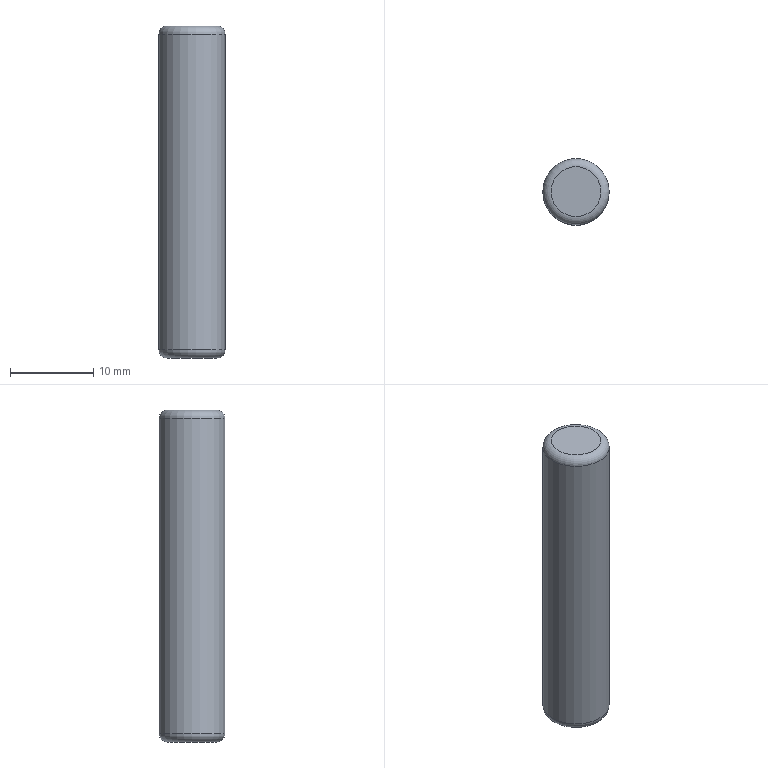Part | STEP file | 1 solid | 5 faces | box 8 x 8 x 40 mm | volume 2000 mm3 | plane 2 | torus 2 | cylinder 1 | commonest cylinder face diameters 8 x1
STEP:
#1=CARTESIAN_POINT('',(0.,0.,0.));
#2=DIRECTION('',(0.,0.,1.));
#3=DIRECTION('',(1.,0.,0.));
#4=AXIS2_PLACEMENT_3D('',#1,#2,#3);
#5=CARTESIAN_POINT('',(1804.247,322.98,18.619));
#6=VERTEX_POINT('',#5);
#7=CARTESIAN_POINT('',(1801.247,322.98,18.619));
#8=DIRECTION('',(0.,0.,-1.));
#9=DIRECTION('',(1.,0.,0.));
#10=AXIS2_PLACEMENT_3D('',#7,#8,#9);
#11=CIRCLE('',#10,3.);
#12=CARTESIAN_POINT('',(1801.247,322.98,18.619));
#13=DIRECTION('',(0.,0.,-1.));
#14=DIRECTION('',(-1.,0.,0.));
#15=AXIS2_PLACEMENT_3D('',#12,#13,#14);
#16=PLANE('',#15);
#17=CARTESIAN_POINT('',(0.,0.));
#18=DIRECTION('',(-1.,0.));
#19=AXIS2_PLACEMENT_2D('',#17,#18);
#20=CIRCLE('',#19,3.);
#21=(GEOMETRIC_REPRESENTATION_CONTEXT(2)PARAMETRIC_REPRESENTATION_CONTEXT()REPRESENTATION_CONTEXT('',''));
#22=DEFINITIONAL_REPRESENTATION('',(#20),#21);
#23=PCURVE('',#16,#22);
#24=CARTESIAN_POINT('',(1801.247,322.98,19.619));
#25=DIRECTION('',(0.,0.,-1.));
#26=DIRECTION('',(-1.,0.,0.));
#27=AXIS2_PLACEMENT_3D('',#24,#25,#26);
#28=TOROIDAL_SURFACE('',#27,3.,1.);
#29=CARTESIAN_POINT('',(3.142,7.854));
#30=DIRECTION('',(1.,0.));
#31=VECTOR('',#30,1.);
#32=LINE('',#29,#31);
#33=(GEOMETRIC_REPRESENTATION_CONTEXT(2)PARAMETRIC_REPRESENTATION_CONTEXT()REPRESENTATION_CONTEXT('',''));
#34=DEFINITIONAL_REPRESENTATION('',(#32),#33);
#35=PCURVE('',#28,#34);
#36=SURFACE_CURVE('',#11,(#23,#35),.PCURVE_S1.);
#37=EDGE_CURVE('',#6,#6,#36,.T.);
#38=ORIENTED_EDGE('',*,*,#37,.T.);
#39=EDGE_LOOP('',(#38));
#40=FACE_BOUND('',#39,.T.);
#41=ADVANCED_FACE('',(#40),#16,.T.);
#42=CARTESIAN_POINT('',(1798.247,322.98,58.619));
#43=VERTEX_POINT('',#42);
#44=CARTESIAN_POINT('',(1801.247,322.98,58.619));
#45=DIRECTION('',(0.,0.,1.));
#46=DIRECTION('',(-1.,0.,0.));
#47=AXIS2_PLACEMENT_3D('',#44,#45,#46);
#48=CIRCLE('',#47,3.);
#49=CARTESIAN_POINT('',(1801.247,322.98,58.619));
#50=DIRECTION('',(0.,0.,1.));
#51=DIRECTION('',(1.,0.,0.));
#52=AXIS2_PLACEMENT_3D('',#49,#50,#51);
#53=PLANE('',#52);
#54=CARTESIAN_POINT('',(0.,0.));
#55=DIRECTION('',(-1.,0.));
#56=AXIS2_PLACEMENT_2D('',#54,#55);
#57=CIRCLE('',#56,3.);
#58=(GEOMETRIC_REPRESENTATION_CONTEXT(2)PARAMETRIC_REPRESENTATION_CONTEXT()REPRESENTATION_CONTEXT('',''));
#59=DEFINITIONAL_REPRESENTATION('',(#57),#58);
#60=PCURVE('',#53,#59);
#61=CARTESIAN_POINT('',(1801.247,322.98,57.619));
#62=DIRECTION('',(0.,0.,1.));
#63=DIRECTION('',(1.,0.,0.));
#64=AXIS2_PLACEMENT_3D('',#61,#62,#63);
#65=TOROIDAL_SURFACE('',#64,3.,1.);
#66=CARTESIAN_POINT('',(3.142,7.854));
#67=DIRECTION('',(1.,0.));
#68=VECTOR('',#67,1.);
#69=LINE('',#66,#68);
#70=(GEOMETRIC_REPRESENTATION_CONTEXT(2)PARAMETRIC_REPRESENTATION_CONTEXT()REPRESENTATION_CONTEXT('',''));
#71=DEFINITIONAL_REPRESENTATION('',(#69),#70);
#72=PCURVE('',#65,#71);
#73=SURFACE_CURVE('',#48,(#60,#72),.PCURVE_S1.);
#74=EDGE_CURVE('',#43,#43,#73,.T.);
#75=ORIENTED_EDGE('',*,*,#74,.T.);
#76=EDGE_LOOP('',(#75));
#77=FACE_BOUND('',#76,.T.);
#78=ADVANCED_FACE('',(#77),#53,.T.);
#79=CARTESIAN_POINT('',(1797.247,322.98,57.619));
#80=VERTEX_POINT('',#79);
#81=CARTESIAN_POINT('',(1801.247,322.98,57.619));
#82=DIRECTION('',(0.,0.,-1.));
#83=DIRECTION('',(-1.,0.,0.));
#84=AXIS2_PLACEMENT_3D('',#81,#82,#83);
#85=CIRCLE('',#84,4.);
#86=CARTESIAN_POINT('',(1801.247,322.98,43.619));
#87=DIRECTION('',(0.,0.,-1.));
#88=DIRECTION('',(-1.,0.,0.));
#89=AXIS2_PLACEMENT_3D('',#86,#87,#88);
#90=CYLINDRICAL_SURFACE('',#89,4.);
#91=CARTESIAN_POINT('',(0.,-14.));
#92=DIRECTION('',(1.,0.));
#93=VECTOR('',#92,1.);
#94=LINE('',#91,#93);
#95=(GEOMETRIC_REPRESENTATION_CONTEXT(2)PARAMETRIC_REPRESENTATION_CONTEXT()REPRESENTATION_CONTEXT('',''));
#96=DEFINITIONAL_REPRESENTATION('',(#94),#95);
#97=PCURVE('',#90,#96);
#98=CARTESIAN_POINT('',(9.425,6.283));
#99=DIRECTION('',(-1.,0.));
#100=VECTOR('',#99,1.);
#101=LINE('',#98,#100);
#102=(GEOMETRIC_REPRESENTATION_CONTEXT(2)PARAMETRIC_REPRESENTATION_CONTEXT()REPRESENTATION_CONTEXT('',''));
#103=DEFINITIONAL_REPRESENTATION('',(#101),#102);
#104=PCURVE('',#65,#103);
#105=SURFACE_CURVE('',#85,(#97,#104),.PCURVE_S1.);
#106=EDGE_CURVE('',#80,#80,#105,.T.);
#107=ORIENTED_EDGE('',*,*,#106,.T.);
#108=CARTESIAN_POINT('',(1797.247,322.98,19.619));
#109=VERTEX_POINT('',#108);
#110=CARTESIAN_POINT('',(1797.247,322.98,57.619));
#111=CARTESIAN_POINT('',(1797.247,322.98,19.619));
#112=B_SPLINE_CURVE_WITH_KNOTS('',1,(#110,#111),.UNSPECIFIED.,.F.,.F.,(2,2),(-14.,24.),.PIECEWISE_BEZIER_KNOTS.);
#113=CARTESIAN_POINT('',(6.283,0.));
#114=DIRECTION('',(0.,1.));
#115=VECTOR('',#114,1.);
#116=LINE('',#113,#115);
#117=(GEOMETRIC_REPRESENTATION_CONTEXT(2)PARAMETRIC_REPRESENTATION_CONTEXT()REPRESENTATION_CONTEXT('',''));
#118=DEFINITIONAL_REPRESENTATION('',(#116),#117);
#119=PCURVE('',#90,#118);
#120=CARTESIAN_POINT('',(0.,0.));
#121=DIRECTION('',(0.,1.));
#122=VECTOR('',#121,1.);
#123=LINE('',#120,#122);
#124=(GEOMETRIC_REPRESENTATION_CONTEXT(2)PARAMETRIC_REPRESENTATION_CONTEXT()REPRESENTATION_CONTEXT('',''));
#125=DEFINITIONAL_REPRESENTATION('',(#123),#124);
#126=PCURVE('',#90,#125);
#127=SEAM_CURVE('',#112,(#119,#126),.PCURVE_S1.);
#128=EDGE_CURVE('',#80,#109,#127,.T.);
#129=ORIENTED_EDGE('',*,*,#128,.T.);
#130=CARTESIAN_POINT('',(1805.247,322.98,19.619));
#131=VERTEX_POINT('',#130);
#132=CARTESIAN_POINT('',(1801.247,322.98,19.619));
#133=DIRECTION('',(0.,0.,1.));
#134=DIRECTION('',(1.,0.,0.));
#135=AXIS2_PLACEMENT_3D('',#132,#133,#134);
#136=CIRCLE('',#135,4.);
#137=CARTESIAN_POINT('',(9.425,24.));
#138=DIRECTION('',(-1.,0.));
#139=VECTOR('',#138,1.);
#140=LINE('',#137,#139);
#141=(GEOMETRIC_REPRESENTATION_CONTEXT(2)PARAMETRIC_REPRESENTATION_CONTEXT()REPRESENTATION_CONTEXT('',''));
#142=DEFINITIONAL_REPRESENTATION('',(#140),#141);
#143=PCURVE('',#90,#142);
#144=CARTESIAN_POINT('',(9.425,6.283));
#145=DIRECTION('',(-1.,0.));
#146=VECTOR('',#145,1.);
#147=LINE('',#144,#146);
#148=(GEOMETRIC_REPRESENTATION_CONTEXT(2)PARAMETRIC_REPRESENTATION_CONTEXT()REPRESENTATION_CONTEXT('',''));
#149=DEFINITIONAL_REPRESENTATION('',(#147),#148);
#150=PCURVE('',#28,#149);
#151=SURFACE_CURVE('',#136,(#143,#150),.PCURVE_S1.);
#152=EDGE_CURVE('',#109,#131,#151,.T.);
#153=ORIENTED_EDGE('',*,*,#152,.T.);
#154=CARTESIAN_POINT('',(1801.247,322.98,19.619));
#155=DIRECTION('',(0.,0.,1.));
#156=DIRECTION('',(1.,0.,0.));
#157=AXIS2_PLACEMENT_3D('',#154,#155,#156);
#158=CIRCLE('',#157,4.);
#159=CARTESIAN_POINT('',(3.142,24.));
#160=DIRECTION('',(-1.,0.));
#161=VECTOR('',#160,1.);
#162=LINE('',#159,#161);
#163=(GEOMETRIC_REPRESENTATION_CONTEXT(2)PARAMETRIC_REPRESENTATION_CONTEXT()REPRESENTATION_CONTEXT('',''));
#164=DEFINITIONAL_REPRESENTATION('',(#162),#163);
#165=PCURVE('',#90,#164);
#166=CARTESIAN_POINT('',(9.425,6.283));
#167=DIRECTION('',(-1.,0.));
#168=VECTOR('',#167,1.);
#169=LINE('',#166,#168);
#170=(GEOMETRIC_REPRESENTATION_CONTEXT(2)PARAMETRIC_REPRESENTATION_CONTEXT()REPRESENTATION_CONTEXT('',''));
#171=DEFINITIONAL_REPRESENTATION('',(#169),#170);
#172=PCURVE('',#28,#171);
#173=SURFACE_CURVE('',#158,(#165,#172),.PCURVE_S1.);
#174=EDGE_CURVE('',#131,#109,#173,.T.);
#175=ORIENTED_EDGE('',*,*,#174,.T.);
#176=ORIENTED_EDGE('',*,*,#128,.F.);
#177=EDGE_LOOP('',(#107,#129,#153,#175,#176));
#178=FACE_BOUND('',#177,.T.);
#179=ADVANCED_FACE('',(#178),#90,.T.);
#180=ORIENTED_EDGE('',*,*,#74,.F.);
#181=CARTESIAN_POINT('',(1797.247,322.98,57.619));
#182=CARTESIAN_POINT('',(1797.247,322.98,57.886));
#183=CARTESIAN_POINT('',(1797.332,322.98,58.147));
#184=CARTESIAN_POINT('',(1797.495,322.98,58.371));
#185=CARTESIAN_POINT('',(1797.719,322.98,58.534));
#186=CARTESIAN_POINT('',(1797.98,322.98,58.619));
#187=CARTESIAN_POINT('',(1798.247,322.98,58.619));
#188=(BOUNDED_CURVE()B_SPLINE_CURVE(6,(#181,#182,#183,#184,#185,#186,#187),.UNSPECIFIED.,.F.,.F.)B_SPLINE_CURVE_WITH_KNOTS((7,7),(0.,1.571),.PIECEWISE_BEZIER_KNOTS.)CURVE()GEOMETRIC_REPRESENTATION_ITEM()RATIONAL_B_SPLINE_CURVE((1.031,1.01,0.9979,0.994,0.9979,1.01,1.031))REPRESENTATION_ITEM(''));
#189=CARTESIAN_POINT('',(3.142,6.283));
#190=DIRECTION('',(0.,1.));
#191=VECTOR('',#190,1.);
#192=LINE('',#189,#191);
#193=(GEOMETRIC_REPRESENTATION_CONTEXT(2)PARAMETRIC_REPRESENTATION_CONTEXT()REPRESENTATION_CONTEXT('',''));
#194=DEFINITIONAL_REPRESENTATION('',(#192),#193);
#195=PCURVE('',#65,#194);
#196=CARTESIAN_POINT('',(9.425,6.283));
#197=DIRECTION('',(0.,1.));
#198=VECTOR('',#197,1.);
#199=LINE('',#196,#198);
#200=(GEOMETRIC_REPRESENTATION_CONTEXT(2)PARAMETRIC_REPRESENTATION_CONTEXT()REPRESENTATION_CONTEXT('',''));
#201=DEFINITIONAL_REPRESENTATION('',(#199),#200);
#202=PCURVE('',#65,#201);
#203=SEAM_CURVE('',#188,(#195,#202),.PCURVE_S1.);
#204=EDGE_CURVE('',#80,#43,#203,.T.);
#205=ORIENTED_EDGE('',*,*,#204,.F.);
#206=ORIENTED_EDGE('',*,*,#106,.F.);
#207=ORIENTED_EDGE('',*,*,#204,.T.);
#208=EDGE_LOOP('',(#180,#205,#206,#207));
#209=FACE_BOUND('',#208,.T.);
#210=ADVANCED_FACE('',(#209),#65,.T.);
#211=ORIENTED_EDGE('',*,*,#37,.F.);
#212=CARTESIAN_POINT('',(1805.247,322.98,19.619));
#213=CARTESIAN_POINT('',(1805.247,322.98,19.352));
#214=CARTESIAN_POINT('',(1805.162,322.98,19.091));
#215=CARTESIAN_POINT('',(1804.999,322.98,18.867));
#216=CARTESIAN_POINT('',(1804.775,322.98,18.704));
#217=CARTESIAN_POINT('',(1804.515,322.98,18.619));
#218=CARTESIAN_POINT('',(1804.247,322.98,18.619));
#219=(BOUNDED_CURVE()B_SPLINE_CURVE(6,(#212,#213,#214,#215,#216,#217,#218),.UNSPECIFIED.,.F.,.F.)B_SPLINE_CURVE_WITH_KNOTS((7,7),(0.,1.571),.PIECEWISE_BEZIER_KNOTS.)CURVE()GEOMETRIC_REPRESENTATION_ITEM()RATIONAL_B_SPLINE_CURVE((1.031,1.01,0.9979,0.994,0.9979,1.01,1.031))REPRESENTATION_ITEM(''));
#220=CARTESIAN_POINT('',(3.142,6.283));
#221=DIRECTION('',(0.,1.));
#222=VECTOR('',#221,1.);
#223=LINE('',#220,#222);
#224=(GEOMETRIC_REPRESENTATION_CONTEXT(2)PARAMETRIC_REPRESENTATION_CONTEXT()REPRESENTATION_CONTEXT('',''));
#225=DEFINITIONAL_REPRESENTATION('',(#223),#224);
#226=PCURVE('',#28,#225);
#227=CARTESIAN_POINT('',(9.425,6.283));
#228=DIRECTION('',(0.,1.));
#229=VECTOR('',#228,1.);
#230=LINE('',#227,#229);
#231=(GEOMETRIC_REPRESENTATION_CONTEXT(2)PARAMETRIC_REPRESENTATION_CONTEXT()REPRESENTATION_CONTEXT('',''));
#232=DEFINITIONAL_REPRESENTATION('',(#230),#231);
#233=PCURVE('',#28,#232);
#234=SEAM_CURVE('',#219,(#226,#233),.PCURVE_S1.);
#235=EDGE_CURVE('',#131,#6,#234,.T.);
#236=ORIENTED_EDGE('',*,*,#235,.F.);
#237=ORIENTED_EDGE('',*,*,#152,.F.);
#238=ORIENTED_EDGE('',*,*,#174,.F.);
#239=ORIENTED_EDGE('',*,*,#235,.T.);
#240=EDGE_LOOP('',(#211,#236,#237,#238,#239));
#241=FACE_BOUND('',#240,.T.);
#242=ADVANCED_FACE('',(#241),#28,.T.);
#243=CLOSED_SHELL('',(#41,#78,#179,#210,#242));
#244=MANIFOLD_SOLID_BREP('',#243);
#245=(LENGTH_UNIT()NAMED_UNIT(*)SI_UNIT(.MILLI.,.METRE.));
#246=UNCERTAINTY_MEASURE_WITH_UNIT(LENGTH_MEASURE(0.00001),#245,'','');
#247=(NAMED_UNIT(*)PLANE_ANGLE_UNIT()SI_UNIT($,.RADIAN.));
#248=(NAMED_UNIT(*)SI_UNIT($,.STERADIAN.)SOLID_ANGLE_UNIT());
#249=(GEOMETRIC_REPRESENTATION_CONTEXT(3)GLOBAL_UNCERTAINTY_ASSIGNED_CONTEXT((#246))GLOBAL_UNIT_ASSIGNED_CONTEXT((#245,#247,#248))REPRESENTATION_CONTEXT('',''));
#250=ADVANCED_BREP_SHAPE_REPRESENTATION('',(#4,#244),#249);